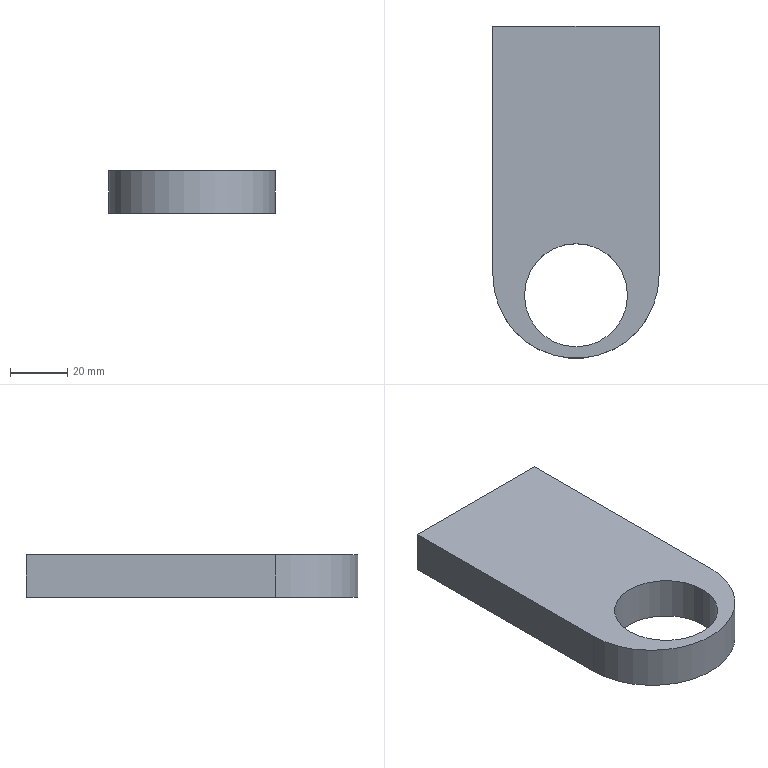Part | SolidWorks | features BaseBody 1 | 1 solid | 8 faces | box 58 x 116 x 15 mm | volume 80237 mm3 | plane 5 | cylinder 3 | commonest cylinder face diameters 36 x2 58 x1
STEP:
#1=CARTESIAN_POINT('',(48.,16.,387.5));
#2=VERTEX_POINT('',#1);
#3=CARTESIAN_POINT('',(12.,16.,387.5));
#4=VERTEX_POINT('',#3);
#5=CARTESIAN_POINT('',(30.,16.,387.5));
#6=DIRECTION('',(0.,0.,-1.));
#7=DIRECTION('',(-1.,0.,0.));
#8=AXIS2_PLACEMENT_3D('',#5,#6,#7);
#9=CIRCLE('',#8,18.);
#10=EDGE_CURVE('',#2,#4,#9,.T.);
#11=ORIENTED_EDGE('',*,*,#10,.F.);
#12=CARTESIAN_POINT('',(48.,16.,372.5));
#13=VERTEX_POINT('',#12);
#14=CARTESIAN_POINT('',(48.,16.,1142.4));
#15=DIRECTION('',(0.,0.,-1.));
#16=VECTOR('',#15,1000.);
#17=LINE('',#14,#16);
#18=EDGE_CURVE('',#2,#13,#17,.T.);
#19=ORIENTED_EDGE('',*,*,#18,.T.);
#20=CARTESIAN_POINT('',(12.,16.,372.5));
#21=VERTEX_POINT('',#20);
#22=CARTESIAN_POINT('',(30.,16.,372.5));
#23=DIRECTION('',(0.,0.,1.));
#24=DIRECTION('',(-1.,0.,0.));
#25=AXIS2_PLACEMENT_3D('',#22,#23,#24);
#26=CIRCLE('',#25,18.);
#27=EDGE_CURVE('',#21,#13,#26,.T.);
#28=ORIENTED_EDGE('',*,*,#27,.F.);
#29=CARTESIAN_POINT('',(12.,16.,1142.4));
#30=DIRECTION('',(0.,0.,-1.));
#31=VECTOR('',#30,1000.);
#32=LINE('',#29,#31);
#33=EDGE_CURVE('',#4,#21,#32,.T.);
#34=ORIENTED_EDGE('',*,*,#33,.F.);
#35=EDGE_LOOP('',(#11,#19,#28,#34));
#36=FACE_OUTER_BOUND('',#35,.T.);
#37=CARTESIAN_POINT('',(30.,16.,1142.4));
#38=DIRECTION('',(0.,0.,-1.));
#39=DIRECTION('',(-1.,0.,0.));
#40=AXIS2_PLACEMENT_3D('',#37,#38,#39);
#41=CYLINDRICAL_SURFACE('',#40,18.);
#42=ADVANCED_FACE('',(#36),#41,.F.);
#43=ORIENTED_EDGE('',*,*,#27,.T.);
#44=CARTESIAN_POINT('',(30.,16.,372.5));
#45=DIRECTION('',(0.,0.,1.));
#46=DIRECTION('',(-1.,0.,0.));
#47=AXIS2_PLACEMENT_3D('',#44,#45,#46);
#48=CIRCLE('',#47,18.);
#49=EDGE_CURVE('',#13,#21,#48,.T.);
#50=ORIENTED_EDGE('',*,*,#49,.T.);
#51=EDGE_LOOP('',(#43,#50));
#52=FACE_BOUND('',#51,.T.);
#53=CARTESIAN_POINT('',(59.,110.,372.5));
#54=VERTEX_POINT('',#53);
#55=CARTESIAN_POINT('',(59.,23.,372.5));
#56=VERTEX_POINT('',#55);
#57=CARTESIAN_POINT('',(59.,21.,372.5));
#58=DIRECTION('',(0.,-1.,0.));
#59=VECTOR('',#58,1000.);
#60=LINE('',#57,#59);
#61=EDGE_CURVE('',#54,#56,#60,.T.);
#62=ORIENTED_EDGE('',*,*,#61,.T.);
#63=CARTESIAN_POINT('',(1.,23.,372.5));
#64=VERTEX_POINT('',#63);
#65=CARTESIAN_POINT('',(30.,23.,372.5));
#66=DIRECTION('',(0.,0.,-1.));
#67=DIRECTION('',(1.,0.,0.));
#68=AXIS2_PLACEMENT_3D('',#65,#66,#67);
#69=CIRCLE('',#68,29.);
#70=EDGE_CURVE('',#56,#64,#69,.T.);
#71=ORIENTED_EDGE('',*,*,#70,.T.);
#72=CARTESIAN_POINT('',(1.,110.,372.5));
#73=VERTEX_POINT('',#72);
#74=CARTESIAN_POINT('',(1.,21.,372.5));
#75=DIRECTION('',(0.,1.,0.));
#76=VECTOR('',#75,1000.);
#77=LINE('',#74,#76);
#78=EDGE_CURVE('',#64,#73,#77,.T.);
#79=ORIENTED_EDGE('',*,*,#78,.T.);
#80=CARTESIAN_POINT('',(30.,110.,372.5));
#81=DIRECTION('',(1.,0.,0.));
#82=VECTOR('',#81,1000.);
#83=LINE('',#80,#82);
#84=EDGE_CURVE('',#73,#54,#83,.T.);
#85=ORIENTED_EDGE('',*,*,#84,.T.);
#86=EDGE_LOOP('',(#62,#71,#79,#85));
#87=FACE_OUTER_BOUND('',#86,.T.);
#88=CARTESIAN_POINT('',(30.,21.,372.5));
#89=DIRECTION('',(0.,0.,-1.));
#90=DIRECTION('',(-1.,0.,0.));
#91=AXIS2_PLACEMENT_3D('',#88,#89,#90);
#92=PLANE('',#91);
#93=ADVANCED_FACE('',(#52,#87),#92,.T.);
#94=ORIENTED_EDGE('',*,*,#18,.F.);
#95=CARTESIAN_POINT('',(30.,16.,387.5));
#96=DIRECTION('',(0.,0.,-1.));
#97=DIRECTION('',(-1.,0.,0.));
#98=AXIS2_PLACEMENT_3D('',#95,#96,#97);
#99=CIRCLE('',#98,18.);
#100=EDGE_CURVE('',#4,#2,#99,.T.);
#101=ORIENTED_EDGE('',*,*,#100,.F.);
#102=ORIENTED_EDGE('',*,*,#33,.T.);
#103=ORIENTED_EDGE('',*,*,#49,.F.);
#104=EDGE_LOOP('',(#94,#101,#102,#103));
#105=FACE_OUTER_BOUND('',#104,.T.);
#106=CARTESIAN_POINT('',(30.,16.,1142.4));
#107=DIRECTION('',(0.,0.,-1.));
#108=DIRECTION('',(-1.,0.,0.));
#109=AXIS2_PLACEMENT_3D('',#106,#107,#108);
#110=CYLINDRICAL_SURFACE('',#109,18.);
#111=ADVANCED_FACE('',(#105),#110,.F.);
#112=CARTESIAN_POINT('',(59.,23.,387.5));
#113=VERTEX_POINT('',#112);
#114=CARTESIAN_POINT('',(59.,23.,372.5));
#115=DIRECTION('',(0.,0.,1.));
#116=VECTOR('',#115,1000.);
#117=LINE('',#114,#116);
#118=EDGE_CURVE('',#56,#113,#117,.T.);
#119=ORIENTED_EDGE('',*,*,#118,.T.);
#120=CARTESIAN_POINT('',(1.,23.,387.5));
#121=VERTEX_POINT('',#120);
#122=CARTESIAN_POINT('',(30.,23.,387.5));
#123=DIRECTION('',(0.,0.,-1.));
#124=DIRECTION('',(1.,0.,0.));
#125=AXIS2_PLACEMENT_3D('',#122,#123,#124);
#126=CIRCLE('',#125,29.);
#127=EDGE_CURVE('',#113,#121,#126,.T.);
#128=ORIENTED_EDGE('',*,*,#127,.T.);
#129=CARTESIAN_POINT('',(1.,23.,372.5));
#130=DIRECTION('',(0.,0.,-1.));
#131=VECTOR('',#130,1000.);
#132=LINE('',#129,#131);
#133=EDGE_CURVE('',#121,#64,#132,.T.);
#134=ORIENTED_EDGE('',*,*,#133,.T.);
#135=ORIENTED_EDGE('',*,*,#70,.F.);
#136=EDGE_LOOP('',(#119,#128,#134,#135));
#137=FACE_OUTER_BOUND('',#136,.T.);
#138=CARTESIAN_POINT('',(30.,23.,372.5));
#139=DIRECTION('',(0.,0.,1.));
#140=DIRECTION('',(1.,0.,0.));
#141=AXIS2_PLACEMENT_3D('',#138,#139,#140);
#142=CYLINDRICAL_SURFACE('',#141,29.);
#143=ADVANCED_FACE('',(#137),#142,.T.);
#144=CARTESIAN_POINT('',(59.,110.,387.5));
#145=VERTEX_POINT('',#144);
#146=CARTESIAN_POINT('',(59.,110.,372.5));
#147=DIRECTION('',(0.,0.,1.));
#148=VECTOR('',#147,1000.);
#149=LINE('',#146,#148);
#150=EDGE_CURVE('',#54,#145,#149,.T.);
#151=ORIENTED_EDGE('',*,*,#150,.T.);
#152=CARTESIAN_POINT('',(59.,21.,387.5));
#153=DIRECTION('',(0.,-1.,0.));
#154=VECTOR('',#153,1000.);
#155=LINE('',#152,#154);
#156=EDGE_CURVE('',#145,#113,#155,.T.);
#157=ORIENTED_EDGE('',*,*,#156,.T.);
#158=ORIENTED_EDGE('',*,*,#118,.F.);
#159=ORIENTED_EDGE('',*,*,#61,.F.);
#160=EDGE_LOOP('',(#151,#157,#158,#159));
#161=FACE_OUTER_BOUND('',#160,.T.);
#162=CARTESIAN_POINT('',(59.,21.,372.5));
#163=DIRECTION('',(1.,0.,0.));
#164=DIRECTION('',(0.,0.,-1.));
#165=AXIS2_PLACEMENT_3D('',#162,#163,#164);
#166=PLANE('',#165);
#167=ADVANCED_FACE('',(#161),#166,.T.);
#168=ORIENTED_EDGE('',*,*,#84,.F.);
#169=CARTESIAN_POINT('',(1.,110.,387.5));
#170=VERTEX_POINT('',#169);
#171=CARTESIAN_POINT('',(1.,110.,407.3));
#172=DIRECTION('',(0.,0.,1.));
#173=VECTOR('',#172,1000.);
#174=LINE('',#171,#173);
#175=EDGE_CURVE('',#73,#170,#174,.T.);
#176=ORIENTED_EDGE('',*,*,#175,.T.);
#177=CARTESIAN_POINT('',(637.958,110.,387.5));
#178=DIRECTION('',(1.,0.,0.));
#179=VECTOR('',#178,1000.);
#180=LINE('',#177,#179);
#181=EDGE_CURVE('',#170,#145,#180,.T.);
#182=ORIENTED_EDGE('',*,*,#181,.T.);
#183=ORIENTED_EDGE('',*,*,#150,.F.);
#184=EDGE_LOOP('',(#168,#176,#182,#183));
#185=FACE_OUTER_BOUND('',#184,.T.);
#186=CARTESIAN_POINT('',(637.958,110.,407.3));
#187=DIRECTION('',(0.,1.,0.));
#188=DIRECTION('',(0.,0.,1.));
#189=AXIS2_PLACEMENT_3D('',#186,#187,#188);
#190=PLANE('',#189);
#191=ADVANCED_FACE('',(#185),#190,.T.);
#192=ORIENTED_EDGE('',*,*,#175,.F.);
#193=ORIENTED_EDGE('',*,*,#78,.F.);
#194=ORIENTED_EDGE('',*,*,#133,.F.);
#195=CARTESIAN_POINT('',(1.,21.,387.5));
#196=DIRECTION('',(0.,1.,0.));
#197=VECTOR('',#196,1000.);
#198=LINE('',#195,#197);
#199=EDGE_CURVE('',#121,#170,#198,.T.);
#200=ORIENTED_EDGE('',*,*,#199,.T.);
#201=EDGE_LOOP('',(#192,#193,#194,#200));
#202=FACE_OUTER_BOUND('',#201,.T.);
#203=CARTESIAN_POINT('',(1.,21.,372.5));
#204=DIRECTION('',(-1.,0.,0.));
#205=DIRECTION('',(0.,0.,1.));
#206=AXIS2_PLACEMENT_3D('',#203,#204,#205);
#207=PLANE('',#206);
#208=ADVANCED_FACE('',(#202),#207,.T.);
#209=ORIENTED_EDGE('',*,*,#100,.T.);
#210=ORIENTED_EDGE('',*,*,#10,.T.);
#211=EDGE_LOOP('',(#209,#210));
#212=FACE_BOUND('',#211,.T.);
#213=ORIENTED_EDGE('',*,*,#181,.F.);
#214=ORIENTED_EDGE('',*,*,#199,.F.);
#215=ORIENTED_EDGE('',*,*,#127,.F.);
#216=ORIENTED_EDGE('',*,*,#156,.F.);
#217=EDGE_LOOP('',(#213,#214,#215,#216));
#218=FACE_OUTER_BOUND('',#217,.T.);
#219=CARTESIAN_POINT('',(30.,21.,387.5));
#220=DIRECTION('',(0.,0.,1.));
#221=DIRECTION('',(1.,0.,0.));
#222=AXIS2_PLACEMENT_3D('',#219,#220,#221);
#223=PLANE('',#222);
#224=ADVANCED_FACE('',(#212,#218),#223,.T.);
#225=CLOSED_SHELL('',(#42,#93,#111,#143,#167,#191,#208,#224));
#226=MANIFOLD_SOLID_BREP('',#225);
#227=CARTESIAN_POINT('',(0.,0.,0.));
#228=DIRECTION('',(0.,0.,1.));
#229=DIRECTION('',(1.,0.,0.));
#230=AXIS2_PLACEMENT_3D('',#227,#228,#229);
#231=(LENGTH_UNIT()NAMED_UNIT(*)SI_UNIT(.MILLI.,.METRE.));
#232=UNCERTAINTY_MEASURE_WITH_UNIT(LENGTH_MEASURE(0.00001),#231,'','');
#233=(NAMED_UNIT(*)PLANE_ANGLE_UNIT()SI_UNIT($,.RADIAN.));
#234=(NAMED_UNIT(*)SI_UNIT($,.STERADIAN.)SOLID_ANGLE_UNIT());
#235=(GEOMETRIC_REPRESENTATION_CONTEXT(3)GLOBAL_UNCERTAINTY_ASSIGNED_CONTEXT((#232))GLOBAL_UNIT_ASSIGNED_CONTEXT((#231,#233,#234))REPRESENTATION_CONTEXT('',''));
#236=ADVANCED_BREP_SHAPE_REPRESENTATION('',(#226,#230),#235);